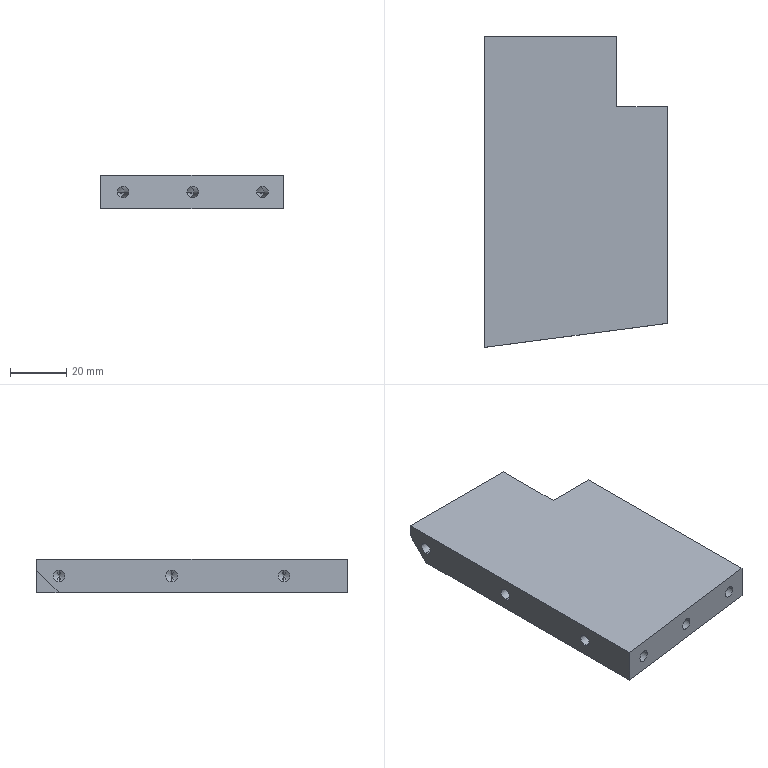Part | SolidWorks | features HoleWzd 4, ICE 3, Extrusion 1 | 1 solid | 46 faces | box 65 x 110.557 x 12 mm | volume 75075 mm3 | cylinder 18 | cone 18 | plane 10 | commonest cylinder face diameters 4.2 x16 4 x2
STEP:
#1=CARTESIAN_POINT('',(6.5,39.5,2.));
#2=VERTEX_POINT('',#1);
#3=CARTESIAN_POINT('',(6.5,39.5,-2.));
#4=VERTEX_POINT('',#3);
#5=CARTESIAN_POINT('',(6.5,39.5,0.));
#6=DIRECTION('',(1.,0.,0.));
#7=DIRECTION('',(0.,0.,-1.));
#8=AXIS2_PLACEMENT_3D('',#5,#6,#7);
#9=CIRCLE('',#8,2.);
#10=EDGE_CURVE('',#2,#4,#9,.T.);
#11=ORIENTED_EDGE('',*,*,#10,.F.);
#12=CARTESIAN_POINT('',(14.5,39.5,2.));
#13=VERTEX_POINT('',#12);
#14=CARTESIAN_POINT('',(14.5,39.5,2.));
#15=DIRECTION('',(1.,0.,0.));
#16=VECTOR('',#15,1000.);
#17=LINE('',#14,#16);
#18=EDGE_CURVE('',#2,#13,#17,.T.);
#19=ORIENTED_EDGE('',*,*,#18,.T.);
#20=CARTESIAN_POINT('',(14.5,39.5,-2.));
#21=VERTEX_POINT('',#20);
#22=CARTESIAN_POINT('',(14.5,39.5,0.));
#23=DIRECTION('',(1.,0.,0.));
#24=DIRECTION('',(0.,0.,-1.));
#25=AXIS2_PLACEMENT_3D('',#22,#23,#24);
#26=CIRCLE('',#25,2.);
#27=EDGE_CURVE('',#13,#21,#26,.T.);
#28=ORIENTED_EDGE('',*,*,#27,.T.);
#29=CARTESIAN_POINT('',(14.5,39.5,-2.));
#30=DIRECTION('',(1.,0.,0.));
#31=VECTOR('',#30,1000.);
#32=LINE('',#29,#31);
#33=EDGE_CURVE('',#4,#21,#32,.T.);
#34=ORIENTED_EDGE('',*,*,#33,.F.);
#35=EDGE_LOOP('',(#11,#19,#28,#34));
#36=FACE_OUTER_BOUND('',#35,.T.);
#37=CARTESIAN_POINT('',(14.5,39.5,0.));
#38=DIRECTION('',(1.,0.,0.));
#39=DIRECTION('',(0.,0.,-1.));
#40=AXIS2_PLACEMENT_3D('',#37,#38,#39);
#41=CYLINDRICAL_SURFACE('',#40,2.);
#42=ADVANCED_FACE('',(#36),#41,.F.);
#43=CARTESIAN_POINT('',(5.298,39.5,0.));
#44=VERTEX_POINT('',#43);
#45=CARTESIAN_POINT('',(6.5,39.5,-2.));
#46=DIRECTION('',(0.515,0.,-0.8572));
#47=VECTOR('',#46,1000.);
#48=LINE('',#45,#47);
#49=EDGE_CURVE('',#44,#4,#48,.T.);
#50=ORIENTED_EDGE('',*,*,#49,.F.);
#51=CARTESIAN_POINT('',(6.5,39.5,2.));
#52=DIRECTION('',(0.515,0.,0.8572));
#53=VECTOR('',#52,1000.);
#54=LINE('',#51,#53);
#55=EDGE_CURVE('',#44,#2,#54,.T.);
#56=ORIENTED_EDGE('',*,*,#55,.T.);
#57=ORIENTED_EDGE('',*,*,#10,.T.);
#58=EDGE_LOOP('',(#50,#56,#57));
#59=FACE_OUTER_BOUND('',#58,.T.);
#60=CARTESIAN_POINT('',(6.5,39.5,0.));
#61=DIRECTION('',(1.,0.,0.));
#62=DIRECTION('',(0.,0.,-1.));
#63=AXIS2_PLACEMENT_3D('',#60,#61,#62);
#64=CONICAL_SURFACE('',#63,2.,1.03);
#65=ADVANCED_FACE('',(#59),#64,.F.);
#66=CARTESIAN_POINT('',(2.1,47.,2.1));
#67=VERTEX_POINT('',#66);
#68=CARTESIAN_POINT('',(2.1,47.,-2.1));
#69=VERTEX_POINT('',#68);
#70=CARTESIAN_POINT('',(2.1,47.,0.));
#71=DIRECTION('',(1.,0.,0.));
#72=DIRECTION('',(0.,0.,-1.));
#73=AXIS2_PLACEMENT_3D('',#70,#71,#72);
#74=CIRCLE('',#73,2.1);
#75=EDGE_CURVE('',#67,#69,#74,.T.);
#76=ORIENTED_EDGE('',*,*,#75,.F.);
#77=CARTESIAN_POINT('',(14.5,47.,2.1));
#78=VERTEX_POINT('',#77);
#79=CARTESIAN_POINT('',(14.5,47.,2.1));
#80=DIRECTION('',(1.,0.,0.));
#81=VECTOR('',#80,1000.);
#82=LINE('',#79,#81);
#83=EDGE_CURVE('',#67,#78,#82,.T.);
#84=ORIENTED_EDGE('',*,*,#83,.T.);
#85=CARTESIAN_POINT('',(14.5,47.,-2.1));
#86=VERTEX_POINT('',#85);
#87=CARTESIAN_POINT('',(14.5,47.,0.));
#88=DIRECTION('',(1.,0.,0.));
#89=DIRECTION('',(0.,0.,-1.));
#90=AXIS2_PLACEMENT_3D('',#87,#88,#89);
#91=CIRCLE('',#90,2.1);
#92=EDGE_CURVE('',#78,#86,#91,.T.);
#93=ORIENTED_EDGE('',*,*,#92,.T.);
#94=CARTESIAN_POINT('',(14.5,47.,-2.1));
#95=DIRECTION('',(1.,0.,0.));
#96=VECTOR('',#95,1000.);
#97=LINE('',#94,#96);
#98=EDGE_CURVE('',#69,#86,#97,.T.);
#99=ORIENTED_EDGE('',*,*,#98,.F.);
#100=EDGE_LOOP('',(#76,#84,#93,#99));
#101=FACE_OUTER_BOUND('',#100,.T.);
#102=CARTESIAN_POINT('',(14.5,47.,0.));
#103=DIRECTION('',(1.,0.,0.));
#104=DIRECTION('',(0.,0.,-1.));
#105=AXIS2_PLACEMENT_3D('',#102,#103,#104);
#106=CYLINDRICAL_SURFACE('',#105,2.1);
#107=ADVANCED_FACE('',(#101),#106,.F.);
#108=CARTESIAN_POINT('',(0.8382,47.,0.));
#109=VERTEX_POINT('',#108);
#110=CARTESIAN_POINT('',(2.1,47.,-2.1));
#111=DIRECTION('',(0.515,0.,-0.8572));
#112=VECTOR('',#111,1000.);
#113=LINE('',#110,#112);
#114=EDGE_CURVE('',#109,#69,#113,.T.);
#115=ORIENTED_EDGE('',*,*,#114,.F.);
#116=CARTESIAN_POINT('',(2.1,47.,2.1));
#117=DIRECTION('',(0.515,0.,0.8572));
#118=VECTOR('',#117,1000.);
#119=LINE('',#116,#118);
#120=EDGE_CURVE('',#109,#67,#119,.T.);
#121=ORIENTED_EDGE('',*,*,#120,.T.);
#122=ORIENTED_EDGE('',*,*,#75,.T.);
#123=EDGE_LOOP('',(#115,#121,#122));
#124=FACE_OUTER_BOUND('',#123,.T.);
#125=CARTESIAN_POINT('',(2.1,47.,0.));
#126=DIRECTION('',(1.,0.,0.));
#127=DIRECTION('',(0.,0.,-1.));
#128=AXIS2_PLACEMENT_3D('',#125,#126,#127);
#129=CONICAL_SURFACE('',#128,2.1,1.03);
#130=ADVANCED_FACE('',(#124),#129,.F.);
#131=CARTESIAN_POINT('',(2.1,32.,2.1));
#132=VERTEX_POINT('',#131);
#133=CARTESIAN_POINT('',(2.1,32.,-2.1));
#134=VERTEX_POINT('',#133);
#135=CARTESIAN_POINT('',(2.1,32.,0.));
#136=DIRECTION('',(1.,0.,0.));
#137=DIRECTION('',(0.,0.,-1.));
#138=AXIS2_PLACEMENT_3D('',#135,#136,#137);
#139=CIRCLE('',#138,2.1);
#140=EDGE_CURVE('',#132,#134,#139,.T.);
#141=ORIENTED_EDGE('',*,*,#140,.F.);
#142=CARTESIAN_POINT('',(14.5,32.,2.1));
#143=VERTEX_POINT('',#142);
#144=CARTESIAN_POINT('',(14.5,32.,2.1));
#145=DIRECTION('',(1.,0.,0.));
#146=VECTOR('',#145,1000.);
#147=LINE('',#144,#146);
#148=EDGE_CURVE('',#132,#143,#147,.T.);
#149=ORIENTED_EDGE('',*,*,#148,.T.);
#150=CARTESIAN_POINT('',(14.5,32.,-2.1));
#151=VERTEX_POINT('',#150);
#152=CARTESIAN_POINT('',(14.5,32.,0.));
#153=DIRECTION('',(1.,0.,0.));
#154=DIRECTION('',(0.,0.,-1.));
#155=AXIS2_PLACEMENT_3D('',#152,#153,#154);
#156=CIRCLE('',#155,2.1);
#157=EDGE_CURVE('',#143,#151,#156,.T.);
#158=ORIENTED_EDGE('',*,*,#157,.T.);
#159=CARTESIAN_POINT('',(14.5,32.,-2.1));
#160=DIRECTION('',(1.,0.,0.));
#161=VECTOR('',#160,1000.);
#162=LINE('',#159,#161);
#163=EDGE_CURVE('',#134,#151,#162,.T.);
#164=ORIENTED_EDGE('',*,*,#163,.F.);
#165=EDGE_LOOP('',(#141,#149,#158,#164));
#166=FACE_OUTER_BOUND('',#165,.T.);
#167=CARTESIAN_POINT('',(14.5,32.,0.));
#168=DIRECTION('',(1.,0.,0.));
#169=DIRECTION('',(0.,0.,-1.));
#170=AXIS2_PLACEMENT_3D('',#167,#168,#169);
#171=CYLINDRICAL_SURFACE('',#170,2.1);
#172=ADVANCED_FACE('',(#166),#171,.F.);
#173=CARTESIAN_POINT('',(0.8382,32.,0.));
#174=VERTEX_POINT('',#173);
#175=CARTESIAN_POINT('',(2.1,32.,-2.1));
#176=DIRECTION('',(0.515,0.,-0.8572));
#177=VECTOR('',#176,1000.);
#178=LINE('',#175,#177);
#179=EDGE_CURVE('',#174,#134,#178,.T.);
#180=ORIENTED_EDGE('',*,*,#179,.F.);
#181=CARTESIAN_POINT('',(2.1,32.,2.1));
#182=DIRECTION('',(0.515,0.,0.8572));
#183=VECTOR('',#182,1000.);
#184=LINE('',#181,#183);
#185=EDGE_CURVE('',#174,#132,#184,.T.);
#186=ORIENTED_EDGE('',*,*,#185,.T.);
#187=ORIENTED_EDGE('',*,*,#140,.T.);
#188=EDGE_LOOP('',(#180,#186,#187));
#189=FACE_OUTER_BOUND('',#188,.T.);
#190=CARTESIAN_POINT('',(2.1,32.,0.));
#191=DIRECTION('',(1.,0.,0.));
#192=DIRECTION('',(0.,0.,-1.));
#193=AXIS2_PLACEMENT_3D('',#190,#191,#192);
#194=CONICAL_SURFACE('',#193,2.1,1.03);
#195=ADVANCED_FACE('',(#189),#194,.F.);
#196=CARTESIAN_POINT('',(-20.1,43.,-2.1));
#197=VERTEX_POINT('',#196);
#198=CARTESIAN_POINT('',(-20.1,43.,2.1));
#199=VERTEX_POINT('',#198);
#200=CARTESIAN_POINT('',(-20.1,43.,0.));
#201=DIRECTION('',(-1.,0.,0.));
#202=DIRECTION('',(0.,0.,1.));
#203=AXIS2_PLACEMENT_3D('',#200,#201,#202);
#204=CIRCLE('',#203,2.1);
#205=EDGE_CURVE('',#197,#199,#204,.T.);
#206=ORIENTED_EDGE('',*,*,#205,.F.);
#207=CARTESIAN_POINT('',(-32.5,43.,-2.1));
#208=VERTEX_POINT('',#207);
#209=CARTESIAN_POINT('',(-32.5,43.,-2.1));
#210=DIRECTION('',(-1.,0.,0.));
#211=VECTOR('',#210,1000.);
#212=LINE('',#209,#211);
#213=EDGE_CURVE('',#197,#208,#212,.T.);
#214=ORIENTED_EDGE('',*,*,#213,.T.);
#215=CARTESIAN_POINT('',(-32.5,43.,2.1));
#216=VERTEX_POINT('',#215);
#217=CARTESIAN_POINT('',(-32.5,43.,0.));
#218=DIRECTION('',(-1.,0.,0.));
#219=DIRECTION('',(0.,0.,1.));
#220=AXIS2_PLACEMENT_3D('',#217,#218,#219);
#221=CIRCLE('',#220,2.1);
#222=EDGE_CURVE('',#208,#216,#221,.T.);
#223=ORIENTED_EDGE('',*,*,#222,.T.);
#224=CARTESIAN_POINT('',(-32.5,43.,2.1));
#225=DIRECTION('',(-1.,0.,0.));
#226=VECTOR('',#225,1000.);
#227=LINE('',#224,#226);
#228=EDGE_CURVE('',#199,#216,#227,.T.);
#229=ORIENTED_EDGE('',*,*,#228,.F.);
#230=EDGE_LOOP('',(#206,#214,#223,#229));
#231=FACE_OUTER_BOUND('',#230,.T.);
#232=CARTESIAN_POINT('',(-32.5,43.,0.));
#233=DIRECTION('',(-1.,0.,0.));
#234=DIRECTION('',(0.,0.,1.));
#235=AXIS2_PLACEMENT_3D('',#232,#233,#234);
#236=CYLINDRICAL_SURFACE('',#235,2.1);
#237=ADVANCED_FACE('',(#231),#236,.F.);
#238=CARTESIAN_POINT('',(-18.838,43.,0.));
#239=VERTEX_POINT('',#238);
#240=CARTESIAN_POINT('',(-20.1,43.,2.1));
#241=DIRECTION('',(-0.515,0.,0.8572));
#242=VECTOR('',#241,1000.);
#243=LINE('',#240,#242);
#244=EDGE_CURVE('',#239,#199,#243,.T.);
#245=ORIENTED_EDGE('',*,*,#244,.F.);
#246=CARTESIAN_POINT('',(-20.1,43.,-2.1));
#247=DIRECTION('',(-0.515,0.,-0.8572));
#248=VECTOR('',#247,1000.);
#249=LINE('',#246,#248);
#250=EDGE_CURVE('',#239,#197,#249,.T.);
#251=ORIENTED_EDGE('',*,*,#250,.T.);
#252=ORIENTED_EDGE('',*,*,#205,.T.);
#253=EDGE_LOOP('',(#245,#251,#252));
#254=FACE_OUTER_BOUND('',#253,.T.);
#255=CARTESIAN_POINT('',(-20.1,43.,0.));
#256=DIRECTION('',(-1.,0.,0.));
#257=DIRECTION('',(0.,0.,1.));
#258=AXIS2_PLACEMENT_3D('',#255,#256,#257);
#259=CONICAL_SURFACE('',#258,2.1,1.03);
#260=ADVANCED_FACE('',(#254),#259,.F.);
#261=CARTESIAN_POINT('',(-20.1,3.,-2.1));
#262=VERTEX_POINT('',#261);
#263=CARTESIAN_POINT('',(-20.1,3.,2.1));
#264=VERTEX_POINT('',#263);
#265=CARTESIAN_POINT('',(-20.1,3.,0.));
#266=DIRECTION('',(-1.,0.,0.));
#267=DIRECTION('',(0.,0.,1.));
#268=AXIS2_PLACEMENT_3D('',#265,#266,#267);
#269=CIRCLE('',#268,2.1);
#270=EDGE_CURVE('',#262,#264,#269,.T.);
#271=ORIENTED_EDGE('',*,*,#270,.F.);
#272=CARTESIAN_POINT('',(-32.5,3.,-2.1));
#273=VERTEX_POINT('',#272);
#274=CARTESIAN_POINT('',(-32.5,3.,-2.1));
#275=DIRECTION('',(-1.,0.,0.));
#276=VECTOR('',#275,1000.);
#277=LINE('',#274,#276);
#278=EDGE_CURVE('',#262,#273,#277,.T.);
#279=ORIENTED_EDGE('',*,*,#278,.T.);
#280=CARTESIAN_POINT('',(-32.5,3.,2.1));
#281=VERTEX_POINT('',#280);
#282=CARTESIAN_POINT('',(-32.5,3.,0.));
#283=DIRECTION('',(-1.,0.,0.));
#284=DIRECTION('',(0.,0.,1.));
#285=AXIS2_PLACEMENT_3D('',#282,#283,#284);
#286=CIRCLE('',#285,2.1);
#287=EDGE_CURVE('',#273,#281,#286,.T.);
#288=ORIENTED_EDGE('',*,*,#287,.T.);
#289=CARTESIAN_POINT('',(-32.5,3.,2.1));
#290=DIRECTION('',(-1.,0.,0.));
#291=VECTOR('',#290,1000.);
#292=LINE('',#289,#291);
#293=EDGE_CURVE('',#264,#281,#292,.T.);
#294=ORIENTED_EDGE('',*,*,#293,.F.);
#295=EDGE_LOOP('',(#271,#279,#288,#294));
#296=FACE_OUTER_BOUND('',#295,.T.);
#297=CARTESIAN_POINT('',(-32.5,3.,0.));
#298=DIRECTION('',(-1.,0.,0.));
#299=DIRECTION('',(0.,0.,1.));
#300=AXIS2_PLACEMENT_3D('',#297,#298,#299);
#301=CYLINDRICAL_SURFACE('',#300,2.1);
#302=ADVANCED_FACE('',(#296),#301,.F.);
#303=CARTESIAN_POINT('',(-18.838,3.,0.));
#304=VERTEX_POINT('',#303);
#305=CARTESIAN_POINT('',(-20.1,3.,2.1));
#306=DIRECTION('',(-0.515,0.,0.8572));
#307=VECTOR('',#306,1000.);
#308=LINE('',#305,#307);
#309=EDGE_CURVE('',#304,#264,#308,.T.);
#310=ORIENTED_EDGE('',*,*,#309,.F.);
#311=CARTESIAN_POINT('',(-20.1,3.,-2.1));
#312=DIRECTION('',(-0.515,0.,-0.8572));
#313=VECTOR('',#312,1000.);
#314=LINE('',#311,#313);
#315=EDGE_CURVE('',#304,#262,#314,.T.);
#316=ORIENTED_EDGE('',*,*,#315,.T.);
#317=ORIENTED_EDGE('',*,*,#270,.T.);
#318=EDGE_LOOP('',(#310,#316,#317));
#319=FACE_OUTER_BOUND('',#318,.T.);
#320=CARTESIAN_POINT('',(-20.1,3.,0.));
#321=DIRECTION('',(-1.,0.,0.));
#322=DIRECTION('',(0.,0.,1.));
#323=AXIS2_PLACEMENT_3D('',#320,#321,#322);
#324=CONICAL_SURFACE('',#323,2.1,1.03);
#325=ADVANCED_FACE('',(#319),#324,.F.);
#326=CARTESIAN_POINT('',(-20.1,-37.,-2.1));
#327=VERTEX_POINT('',#326);
#328=CARTESIAN_POINT('',(-20.1,-37.,2.1));
#329=VERTEX_POINT('',#328);
#330=CARTESIAN_POINT('',(-20.1,-37.,0.));
#331=DIRECTION('',(-1.,0.,0.));
#332=DIRECTION('',(0.,0.,1.));
#333=AXIS2_PLACEMENT_3D('',#330,#331,#332);
#334=CIRCLE('',#333,2.1);
#335=EDGE_CURVE('',#327,#329,#334,.T.);
#336=ORIENTED_EDGE('',*,*,#335,.F.);
#337=CARTESIAN_POINT('',(-32.5,-37.,-2.1));
#338=VERTEX_POINT('',#337);
#339=CARTESIAN_POINT('',(-32.5,-37.,-2.1));
#340=DIRECTION('',(-1.,0.,0.));
#341=VECTOR('',#340,1000.);
#342=LINE('',#339,#341);
#343=EDGE_CURVE('',#327,#338,#342,.T.);
#344=ORIENTED_EDGE('',*,*,#343,.T.);
#345=CARTESIAN_POINT('',(-32.5,-37.,2.1));
#346=VERTEX_POINT('',#345);
#347=CARTESIAN_POINT('',(-32.5,-37.,0.));
#348=DIRECTION('',(-1.,0.,0.));
#349=DIRECTION('',(0.,0.,1.));
#350=AXIS2_PLACEMENT_3D('',#347,#348,#349);
#351=CIRCLE('',#350,2.1);
#352=EDGE_CURVE('',#338,#346,#351,.T.);
#353=ORIENTED_EDGE('',*,*,#352,.T.);
#354=CARTESIAN_POINT('',(-32.5,-37.,2.1));
#355=DIRECTION('',(-1.,0.,0.));
#356=VECTOR('',#355,1000.);
#357=LINE('',#354,#356);
#358=EDGE_CURVE('',#329,#346,#357,.T.);
#359=ORIENTED_EDGE('',*,*,#358,.F.);
#360=EDGE_LOOP('',(#336,#344,#353,#359));
#361=FACE_OUTER_BOUND('',#360,.T.);
#362=CARTESIAN_POINT('',(-32.5,-37.,0.));
#363=DIRECTION('',(-1.,0.,0.));
#364=DIRECTION('',(0.,0.,1.));
#365=AXIS2_PLACEMENT_3D('',#362,#363,#364);
#366=CYLINDRICAL_SURFACE('',#365,2.1);
#367=ADVANCED_FACE('',(#361),#366,.F.);
#368=CARTESIAN_POINT('',(-18.838,-37.,0.));
#369=VERTEX_POINT('',#368);
#370=CARTESIAN_POINT('',(-20.1,-37.,2.1));
#371=DIRECTION('',(-0.515,0.,0.8572));
#372=VECTOR('',#371,1000.);
#373=LINE('',#370,#372);
#374=EDGE_CURVE('',#369,#329,#373,.T.);
#375=ORIENTED_EDGE('',*,*,#374,.F.);
#376=CARTESIAN_POINT('',(-20.1,-37.,-2.1));
#377=DIRECTION('',(-0.515,0.,-0.8572));
#378=VECTOR('',#377,1000.);
#379=LINE('',#376,#378);
#380=EDGE_CURVE('',#369,#327,#379,.T.);
#381=ORIENTED_EDGE('',*,*,#380,.T.);
#382=ORIENTED_EDGE('',*,*,#335,.T.);
#383=EDGE_LOOP('',(#375,#381,#382));
#384=FACE_OUTER_BOUND('',#383,.T.);
#385=CARTESIAN_POINT('',(-20.1,-37.,0.));
#386=DIRECTION('',(-1.,0.,0.));
#387=DIRECTION('',(0.,0.,1.));
#388=AXIS2_PLACEMENT_3D('',#385,#386,#387);
#389=CONICAL_SURFACE('',#388,2.1,1.03);
#390=ADVANCED_FACE('',(#384),#389,.F.);
#391=CARTESIAN_POINT('',(21.364,-39.959,0.));
#392=VERTEX_POINT('',#391);
#393=CARTESIAN_POINT('',(25.528,-39.411,0.));
#394=VERTEX_POINT('',#393);
#395=CARTESIAN_POINT('',(23.446,-39.685,0.));
#396=DIRECTION('',(0.1305,-0.9914,0.));
#397=DIRECTION('',(0.9914,0.1305,0.));
#398=AXIS2_PLACEMENT_3D('',#395,#396,#397);
#399=CIRCLE('',#398,2.1);
#400=EDGE_CURVE('',#392,#394,#399,.T.);
#401=ORIENTED_EDGE('',*,*,#400,.F.);
#402=CARTESIAN_POINT('',(22.982,-52.253,0.));
#403=VERTEX_POINT('',#402);
#404=CARTESIAN_POINT('',(22.982,-52.253,0.));
#405=DIRECTION('',(0.1305,-0.9914,0.));
#406=VECTOR('',#405,1000.);
#407=LINE('',#404,#406);
#408=EDGE_CURVE('',#392,#403,#407,.T.);
#409=ORIENTED_EDGE('',*,*,#408,.T.);
#410=CARTESIAN_POINT('',(27.146,-51.705,0.));
#411=VERTEX_POINT('',#410);
#412=CARTESIAN_POINT('',(25.064,-51.979,0.));
#413=DIRECTION('',(0.1305,-0.9914,0.));
#414=DIRECTION('',(0.9914,0.1305,0.));
#415=AXIS2_PLACEMENT_3D('',#412,#413,#414);
#416=CIRCLE('',#415,2.1);
#417=EDGE_CURVE('',#403,#411,#416,.T.);
#418=ORIENTED_EDGE('',*,*,#417,.T.);
#419=CARTESIAN_POINT('',(27.146,-51.705,0.));
#420=DIRECTION('',(0.1305,-0.9914,0.));
#421=VECTOR('',#420,1000.);
#422=LINE('',#419,#421);
#423=EDGE_CURVE('',#394,#411,#422,.T.);
#424=ORIENTED_EDGE('',*,*,#423,.F.);
#425=EDGE_LOOP('',(#401,#409,#418,#424));
#426=FACE_OUTER_BOUND('',#425,.T.);
#427=CARTESIAN_POINT('',(25.064,-51.979,0.));
#428=DIRECTION('',(0.1305,-0.9914,0.));
#429=DIRECTION('',(0.9914,0.1305,0.));
#430=AXIS2_PLACEMENT_3D('',#427,#428,#429);
#431=CYLINDRICAL_SURFACE('',#430,2.1);
#432=ADVANCED_FACE('',(#426),#431,.F.);
#433=CARTESIAN_POINT('',(23.281,-38.434,0.));
#434=VERTEX_POINT('',#433);
#435=CARTESIAN_POINT('',(25.528,-39.411,0.));
#436=DIRECTION('',(0.9171,-0.3987,0.));
#437=VECTOR('',#436,1000.);
#438=LINE('',#435,#437);
#439=EDGE_CURVE('',#434,#394,#438,.T.);
#440=ORIENTED_EDGE('',*,*,#439,.F.);
#441=CARTESIAN_POINT('',(21.364,-39.959,0.));
#442=DIRECTION('',(-0.7826,-0.6225,0.));
#443=VECTOR('',#442,1000.);
#444=LINE('',#441,#443);
#445=EDGE_CURVE('',#434,#392,#444,.T.);
#446=ORIENTED_EDGE('',*,*,#445,.T.);
#447=ORIENTED_EDGE('',*,*,#400,.T.);
#448=EDGE_LOOP('',(#440,#446,#447));
#449=FACE_OUTER_BOUND('',#448,.T.);
#450=CARTESIAN_POINT('',(23.446,-39.685,0.));
#451=DIRECTION('',(0.1305,-0.9914,0.));
#452=DIRECTION('',(0.9914,0.1305,0.));
#453=AXIS2_PLACEMENT_3D('',#450,#451,#452);
#454=CONICAL_SURFACE('',#453,2.1,1.03);
#455=ADVANCED_FACE('',(#449),#454,.F.);
#456=CARTESIAN_POINT('',(-3.423,-43.222,0.));
#457=VERTEX_POINT('',#456);
#458=CARTESIAN_POINT('',(0.7416,-42.674,0.));
#459=VERTEX_POINT('',#458);
#460=CARTESIAN_POINT('',(-1.34,-42.948,0.));
#461=DIRECTION('',(0.1305,-0.9914,0.));
#462=DIRECTION('',(0.9914,0.1305,0.));
#463=AXIS2_PLACEMENT_3D('',#460,#461,#462);
#464=CIRCLE('',#463,2.1);
#465=EDGE_CURVE('',#457,#459,#464,.T.);
#466=ORIENTED_EDGE('',*,*,#465,.F.);
#467=CARTESIAN_POINT('',(-1.804,-55.516,0.));
#468=VERTEX_POINT('',#467);
#469=CARTESIAN_POINT('',(-1.804,-55.516,0.));
#470=DIRECTION('',(0.1305,-0.9914,0.));
#471=VECTOR('',#470,1000.);
#472=LINE('',#469,#471);
#473=EDGE_CURVE('',#457,#468,#472,.T.);
#474=ORIENTED_EDGE('',*,*,#473,.T.);
#475=CARTESIAN_POINT('',(2.36,-54.968,0.));
#476=VERTEX_POINT('',#475);
#477=CARTESIAN_POINT('',(0.278,-55.242,0.));
#478=DIRECTION('',(0.1305,-0.9914,0.));
#479=DIRECTION('',(0.9914,0.1305,0.));
#480=AXIS2_PLACEMENT_3D('',#477,#478,#479);
#481=CIRCLE('',#480,2.1);
#482=EDGE_CURVE('',#468,#476,#481,.T.);
#483=ORIENTED_EDGE('',*,*,#482,.T.);
#484=CARTESIAN_POINT('',(2.36,-54.968,0.));
#485=DIRECTION('',(0.1305,-0.9914,0.));
#486=VECTOR('',#485,1000.);
#487=LINE('',#484,#486);
#488=EDGE_CURVE('',#459,#476,#487,.T.);
#489=ORIENTED_EDGE('',*,*,#488,.F.);
#490=EDGE_LOOP('',(#466,#474,#483,#489));
#491=FACE_OUTER_BOUND('',#490,.T.);
#492=CARTESIAN_POINT('',(0.278,-55.242,0.));
#493=DIRECTION('',(0.1305,-0.9914,0.));
#494=DIRECTION('',(0.9914,0.1305,0.));
#495=AXIS2_PLACEMENT_3D('',#492,#493,#494);
#496=CYLINDRICAL_SURFACE('',#495,2.1);
#497=ADVANCED_FACE('',(#491),#496,.F.);
#498=CARTESIAN_POINT('',(-1.505,-41.697,0.));
#499=VERTEX_POINT('',#498);
#500=CARTESIAN_POINT('',(0.7416,-42.674,0.));
#501=DIRECTION('',(0.9171,-0.3987,0.));
#502=VECTOR('',#501,1000.);
#503=LINE('',#500,#502);
#504=EDGE_CURVE('',#499,#459,#503,.T.);
#505=ORIENTED_EDGE('',*,*,#504,.F.);
#506=CARTESIAN_POINT('',(-3.423,-43.222,0.));
#507=DIRECTION('',(-0.7826,-0.6225,0.));
#508=VECTOR('',#507,1000.);
#509=LINE('',#506,#508);
#510=EDGE_CURVE('',#499,#457,#509,.T.);
#511=ORIENTED_EDGE('',*,*,#510,.T.);
#512=ORIENTED_EDGE('',*,*,#465,.T.);
#513=EDGE_LOOP('',(#505,#511,#512));
#514=FACE_OUTER_BOUND('',#513,.T.);
#515=CARTESIAN_POINT('',(-1.34,-42.948,0.));
#516=DIRECTION('',(0.1305,-0.9914,0.));
#517=DIRECTION('',(0.9914,0.1305,0.));
#518=AXIS2_PLACEMENT_3D('',#515,#516,#517);
#519=CONICAL_SURFACE('',#518,2.1,1.03);
#520=ADVANCED_FACE('',(#514),#519,.F.);
#521=CARTESIAN_POINT('',(-28.209,-46.485,0.));
#522=VERTEX_POINT('',#521);
#523=CARTESIAN_POINT('',(-24.045,-45.937,0.));
#524=VERTEX_POINT('',#523);
#525=CARTESIAN_POINT('',(-26.127,-46.211,0.));
#526=DIRECTION('',(0.1305,-0.9914,0.));
#527=DIRECTION('',(0.9914,0.1305,0.));
#528=AXIS2_PLACEMENT_3D('',#525,#526,#527);
#529=CIRCLE('',#528,2.1);
#530=EDGE_CURVE('',#522,#524,#529,.T.);
#531=ORIENTED_EDGE('',*,*,#530,.F.);
#532=CARTESIAN_POINT('',(-26.59,-58.779,0.));
#533=VERTEX_POINT('',#532);
#534=CARTESIAN_POINT('',(-26.59,-58.779,0.));
#535=DIRECTION('',(0.1305,-0.9914,0.));
#536=VECTOR('',#535,1000.);
#537=LINE('',#534,#536);
#538=EDGE_CURVE('',#522,#533,#537,.T.);
#539=ORIENTED_EDGE('',*,*,#538,.T.);
#540=CARTESIAN_POINT('',(-22.426,-58.231,0.));
#541=VERTEX_POINT('',#540);
#542=CARTESIAN_POINT('',(-24.508,-58.505,0.));
#543=DIRECTION('',(0.1305,-0.9914,0.));
#544=DIRECTION('',(0.9914,0.1305,0.));
#545=AXIS2_PLACEMENT_3D('',#542,#543,#544);
#546=CIRCLE('',#545,2.1);
#547=EDGE_CURVE('',#533,#541,#546,.T.);
#548=ORIENTED_EDGE('',*,*,#547,.T.);
#549=CARTESIAN_POINT('',(-22.426,-58.231,0.));
#550=DIRECTION('',(0.1305,-0.9914,0.));
#551=VECTOR('',#550,1000.);
#552=LINE('',#549,#551);
#553=EDGE_CURVE('',#524,#541,#552,.T.);
#554=ORIENTED_EDGE('',*,*,#553,.F.);
#555=EDGE_LOOP('',(#531,#539,#548,#554));
#556=FACE_OUTER_BOUND('',#555,.T.);
#557=CARTESIAN_POINT('',(-24.508,-58.505,0.));
#558=DIRECTION('',(0.1305,-0.9914,0.));
#559=DIRECTION('',(0.9914,0.1305,0.));
#560=AXIS2_PLACEMENT_3D('',#557,#558,#559);
#561=CYLINDRICAL_SURFACE('',#560,2.1);
#562=ADVANCED_FACE('',(#556),#561,.F.);
#563=CARTESIAN_POINT('',(-26.291,-44.96,0.));
#564=VERTEX_POINT('',#563);
#565=CARTESIAN_POINT('',(-24.045,-45.937,0.));
#566=DIRECTION('',(0.9171,-0.3987,0.));
#567=VECTOR('',#566,1000.);
#568=LINE('',#565,#567);
#569=EDGE_CURVE('',#564,#524,#568,.T.);
#570=ORIENTED_EDGE('',*,*,#569,.F.);
#571=CARTESIAN_POINT('',(-28.209,-46.485,0.));
#572=DIRECTION('',(-0.7826,-0.6225,0.));
#573=VECTOR('',#572,1000.);
#574=LINE('',#571,#573);
#575=EDGE_CURVE('',#564,#522,#574,.T.);
#576=ORIENTED_EDGE('',*,*,#575,.T.);
#577=ORIENTED_EDGE('',*,*,#530,.T.);
#578=EDGE_LOOP('',(#570,#576,#577));
#579=FACE_OUTER_BOUND('',#578,.T.);
#580=CARTESIAN_POINT('',(-26.127,-46.211,0.));
#581=DIRECTION('',(0.1305,-0.9914,0.));
#582=DIRECTION('',(0.9914,0.1305,0.));
#583=AXIS2_PLACEMENT_3D('',#580,#581,#582);
#584=CONICAL_SURFACE('',#583,2.1,1.03);
#585=ADVANCED_FACE('',(#579),#584,.F.);
#586=CARTESIAN_POINT('',(32.5,26.,-6.));
#587=VERTEX_POINT('',#586);
#588=CARTESIAN_POINT('',(32.5,-51.,-6.));
#589=VERTEX_POINT('',#588);
#590=CARTESIAN_POINT('',(32.5,51.,-6.));
#591=DIRECTION('',(0.,-1.,0.));
#592=VECTOR('',#591,1000.);
#593=LINE('',#590,#592);
#594=EDGE_CURVE('',#587,#589,#593,.T.);
#595=ORIENTED_EDGE('',*,*,#594,.F.);
#596=CARTESIAN_POINT('',(32.5,26.,6.));
#597=VERTEX_POINT('',#596);
#598=CARTESIAN_POINT('',(32.5,26.,-6.));
#599=DIRECTION('',(0.,0.,1.));
#600=VECTOR('',#599,1000.);
#601=LINE('',#598,#600);
#602=EDGE_CURVE('',#587,#597,#601,.T.);
#603=ORIENTED_EDGE('',*,*,#602,.T.);
#604=CARTESIAN_POINT('',(32.5,-51.,6.));
#605=VERTEX_POINT('',#604);
#606=CARTESIAN_POINT('',(32.5,51.,6.));
#607=DIRECTION('',(0.,-1.,0.));
#608=VECTOR('',#607,1000.);
#609=LINE('',#606,#608);
#610=EDGE_CURVE('',#597,#605,#609,.T.);
#611=ORIENTED_EDGE('',*,*,#610,.T.);
#612=CARTESIAN_POINT('',(32.5,-51.,-6.));
#613=DIRECTION('',(0.,0.,-1.));
#614=VECTOR('',#613,1000.);
#615=LINE('',#612,#614);
#616=EDGE_CURVE('',#605,#589,#615,.T.);
#617=ORIENTED_EDGE('',*,*,#616,.T.);
#618=EDGE_LOOP('',(#595,#603,#611,#617));
#619=FACE_OUTER_BOUND('',#618,.T.);
#620=CARTESIAN_POINT('',(32.5,51.,-6.));
#621=DIRECTION('',(-1.,0.,0.));
#622=DIRECTION('',(0.,0.,1.));
#623=AXIS2_PLACEMENT_3D('',#620,#621,#622);
#624=PLANE('',#623);
#625=ADVANCED_FACE('',(#619),#624,.F.);
#626=CARTESIAN_POINT('',(-32.5,43.,-6.));
#627=VERTEX_POINT('',#626);
#628=CARTESIAN_POINT('',(-32.5,-59.557,-6.));
#629=VERTEX_POINT('',#628);
#630=CARTESIAN_POINT('',(-32.5,51.,-6.));
#631=DIRECTION('',(0.,-1.,0.));
#632=VECTOR('',#631,1000.);
#633=LINE('',#630,#632);
#634=EDGE_CURVE('',#627,#629,#633,.T.);
#635=ORIENTED_EDGE('',*,*,#634,.F.);
#636=CARTESIAN_POINT('',(-4.5,43.,-6.));
#637=VERTEX_POINT('',#636);
#638=CARTESIAN_POINT('',(-4.5,43.,-6.));
#639=DIRECTION('',(-1.,0.,0.));
#640=VECTOR('',#639,1000.);
#641=LINE('',#638,#640);
#642=EDGE_CURVE('',#637,#627,#641,.T.);
#643=ORIENTED_EDGE('',*,*,#642,.F.);
#644=CARTESIAN_POINT('',(-4.5,51.,-6.));
#645=VERTEX_POINT('',#644);
#646=CARTESIAN_POINT('',(-4.5,43.,-6.));
#647=DIRECTION('',(0.,-1.,0.));
#648=VECTOR('',#647,1000.);
#649=LINE('',#646,#648);
#650=EDGE_CURVE('',#645,#637,#649,.T.);
#651=ORIENTED_EDGE('',*,*,#650,.F.);
#652=CARTESIAN_POINT('',(14.5,51.,-6.));
#653=VERTEX_POINT('',#652);
#654=CARTESIAN_POINT('',(-32.5,51.,-6.));
#655=DIRECTION('',(-1.,0.,0.));
#656=VECTOR('',#655,1000.);
#657=LINE('',#654,#656);
#658=EDGE_CURVE('',#653,#645,#657,.T.);
#659=ORIENTED_EDGE('',*,*,#658,.F.);
#660=CARTESIAN_POINT('',(14.5,26.,-6.));
#661=VERTEX_POINT('',#660);
#662=CARTESIAN_POINT('',(14.5,51.,-6.));
#663=DIRECTION('',(0.,-1.,0.));
#664=VECTOR('',#663,1000.);
#665=LINE('',#662,#664);
#666=EDGE_CURVE('',#653,#661,#665,.T.);
#667=ORIENTED_EDGE('',*,*,#666,.T.);
#668=CARTESIAN_POINT('',(32.5,26.,-6.));
#669=DIRECTION('',(1.,0.,0.));
#670=VECTOR('',#669,1000.);
#671=LINE('',#668,#670);
#672=EDGE_CURVE('',#661,#587,#671,.T.);
#673=ORIENTED_EDGE('',*,*,#672,.T.);
#674=ORIENTED_EDGE('',*,*,#594,.T.);
#675=CARTESIAN_POINT('',(32.5,-51.,-6.));
#676=DIRECTION('',(-0.9914,-0.1305,0.));
#677=VECTOR('',#676,1000.);
#678=LINE('',#675,#677);
#679=EDGE_CURVE('',#589,#629,#678,.T.);
#680=ORIENTED_EDGE('',*,*,#679,.T.);
#681=EDGE_LOOP('',(#635,#643,#651,#659,#667,#673,#674,#680));
#682=FACE_OUTER_BOUND('',#681,.T.);
#683=CARTESIAN_POINT('',(-32.5,51.,-6.));
#684=DIRECTION('',(0.,0.,1.));
#685=DIRECTION('',(1.,0.,0.));
#686=AXIS2_PLACEMENT_3D('',#683,#684,#685);
#687=PLANE('',#686);
#688=ADVANCED_FACE('',(#682),#687,.F.);
#689=CARTESIAN_POINT('',(-32.5,43.,0.));
#690=DIRECTION('',(-1.,0.,0.));
#691=DIRECTION('',(0.,0.,1.));
#692=AXIS2_PLACEMENT_3D('',#689,#690,#691);
#693=CIRCLE('',#692,2.1);
#694=EDGE_CURVE('',#216,#208,#693,.T.);
#695=ORIENTED_EDGE('',*,*,#694,.F.);
#696=ORIENTED_EDGE('',*,*,#222,.F.);
#697=EDGE_LOOP('',(#695,#696));
#698=FACE_BOUND('',#697,.T.);
#699=CARTESIAN_POINT('',(-32.5,3.,0.));
#700=DIRECTION('',(-1.,0.,0.));
#701=DIRECTION('',(0.,0.,1.));
#702=AXIS2_PLACEMENT_3D('',#699,#700,#701);
#703=CIRCLE('',#702,2.1);
#704=EDGE_CURVE('',#281,#273,#703,.T.);
#705=ORIENTED_EDGE('',*,*,#704,.F.);
#706=ORIENTED_EDGE('',*,*,#287,.F.);
#707=EDGE_LOOP('',(#705,#706));
#708=FACE_BOUND('',#707,.T.);
#709=CARTESIAN_POINT('',(-32.5,-37.,0.));
#710=DIRECTION('',(-1.,0.,0.));
#711=DIRECTION('',(0.,0.,1.));
#712=AXIS2_PLACEMENT_3D('',#709,#710,#711);
#713=CIRCLE('',#712,2.1);
#714=EDGE_CURVE('',#346,#338,#713,.T.);
#715=ORIENTED_EDGE('',*,*,#714,.F.);
#716=ORIENTED_EDGE('',*,*,#352,.F.);
#717=EDGE_LOOP('',(#715,#716));
#718=FACE_BOUND('',#717,.T.);
#719=CARTESIAN_POINT('',(-32.5,51.,2.));
#720=VERTEX_POINT('',#719);
#721=CARTESIAN_POINT('',(-32.5,51.,6.));
#722=VERTEX_POINT('',#721);
#723=CARTESIAN_POINT('',(-32.5,51.,-6.));
#724=DIRECTION('',(0.,0.,1.));
#725=VECTOR('',#724,1000.);
#726=LINE('',#723,#725);
#727=EDGE_CURVE('',#720,#722,#726,.T.);
#728=ORIENTED_EDGE('',*,*,#727,.F.);
#729=CARTESIAN_POINT('',(-32.5,51.,2.));
#730=DIRECTION('',(0.,0.7071,0.7071));
#731=VECTOR('',#730,1000.);
#732=LINE('',#729,#731);
#733=EDGE_CURVE('',#627,#720,#732,.T.);
#734=ORIENTED_EDGE('',*,*,#733,.F.);
#735=ORIENTED_EDGE('',*,*,#634,.T.);
#736=CARTESIAN_POINT('',(-32.5,-59.557,6.));
#737=VERTEX_POINT('',#736);
#738=CARTESIAN_POINT('',(-32.5,-59.557,-71.561));
#739=DIRECTION('',(0.,0.,1.));
#740=VECTOR('',#739,1000.);
#741=LINE('',#738,#740);
#742=EDGE_CURVE('',#629,#737,#741,.T.);
#743=ORIENTED_EDGE('',*,*,#742,.T.);
#744=CARTESIAN_POINT('',(-32.5,51.,6.));
#745=DIRECTION('',(0.,-1.,0.));
#746=VECTOR('',#745,1000.);
#747=LINE('',#744,#746);
#748=EDGE_CURVE('',#722,#737,#747,.T.);
#749=ORIENTED_EDGE('',*,*,#748,.F.);
#750=EDGE_LOOP('',(#728,#734,#735,#743,#749));
#751=FACE_OUTER_BOUND('',#750,.T.);
#752=CARTESIAN_POINT('',(-32.5,51.,-6.));
#753=DIRECTION('',(1.,0.,0.));
#754=DIRECTION('',(0.,0.,-1.));
#755=AXIS2_PLACEMENT_3D('',#752,#753,#754);
#756=PLANE('',#755);
#757=ADVANCED_FACE('',(#698,#708,#718,#751),#756,.F.);
#758=ORIENTED_EDGE('',*,*,#610,.F.);
#759=CARTESIAN_POINT('',(14.5,26.,6.));
#760=VERTEX_POINT('',#759);
#761=CARTESIAN_POINT('',(32.5,26.,6.));
#762=DIRECTION('',(1.,0.,0.));
#763=VECTOR('',#762,1000.);
#764=LINE('',#761,#763);
#765=EDGE_CURVE('',#760,#597,#764,.T.);
#766=ORIENTED_EDGE('',*,*,#765,.F.);
#767=CARTESIAN_POINT('',(14.5,51.,6.));
#768=VERTEX_POINT('',#767);
#769=CARTESIAN_POINT('',(14.5,51.,6.));
#770=DIRECTION('',(0.,-1.,0.));
#771=VECTOR('',#770,1000.);
#772=LINE('',#769,#771);
#773=EDGE_CURVE('',#768,#760,#772,.T.);
#774=ORIENTED_EDGE('',*,*,#773,.F.);
#775=CARTESIAN_POINT('',(-32.5,51.,6.));
#776=DIRECTION('',(1.,0.,0.));
#777=VECTOR('',#776,1000.);
#778=LINE('',#775,#777);
#779=EDGE_CURVE('',#722,#768,#778,.T.);
#780=ORIENTED_EDGE('',*,*,#779,.F.);
#781=ORIENTED_EDGE('',*,*,#748,.T.);
#782=CARTESIAN_POINT('',(32.5,-51.,6.));
#783=DIRECTION('',(0.9914,0.1305,0.));
#784=VECTOR('',#783,1000.);
#785=LINE('',#782,#784);
#786=EDGE_CURVE('',#737,#605,#785,.T.);
#787=ORIENTED_EDGE('',*,*,#786,.T.);
#788=EDGE_LOOP('',(#758,#766,#774,#780,#781,#787));
#789=FACE_OUTER_BOUND('',#788,.T.);
#790=CARTESIAN_POINT('',(-32.5,51.,6.));
#791=DIRECTION('',(0.,0.,-1.));
#792=DIRECTION('',(-1.,0.,0.));
#793=AXIS2_PLACEMENT_3D('',#790,#791,#792);
#794=PLANE('',#793);
#795=ADVANCED_FACE('',(#789),#794,.F.);
#796=CARTESIAN_POINT('',(-4.5,51.,2.));
#797=VERTEX_POINT('',#796);
#798=CARTESIAN_POINT('',(-4.5,51.,2.));
#799=DIRECTION('',(-1.,0.,0.));
#800=VECTOR('',#799,1000.);
#801=LINE('',#798,#800);
#802=EDGE_CURVE('',#797,#720,#801,.T.);
#803=ORIENTED_EDGE('',*,*,#802,.T.);
#804=ORIENTED_EDGE('',*,*,#727,.T.);
#805=ORIENTED_EDGE('',*,*,#779,.T.);
#806=CARTESIAN_POINT('',(14.5,51.,-6.));
#807=DIRECTION('',(0.,0.,1.));
#808=VECTOR('',#807,1000.);
#809=LINE('',#806,#808);
#810=EDGE_CURVE('',#653,#768,#809,.T.);
#811=ORIENTED_EDGE('',*,*,#810,.F.);
#812=ORIENTED_EDGE('',*,*,#658,.T.);
#813=CARTESIAN_POINT('',(-4.5,51.,-6.));
#814=DIRECTION('',(0.,0.,-1.));
#815=VECTOR('',#814,1000.);
#816=LINE('',#813,#815);
#817=EDGE_CURVE('',#797,#645,#816,.T.);
#818=ORIENTED_EDGE('',*,*,#817,.F.);
#819=EDGE_LOOP('',(#803,#804,#805,#811,#812,#818));
#820=FACE_OUTER_BOUND('',#819,.T.);
#821=CARTESIAN_POINT('',(0.,51.,0.));
#822=DIRECTION('',(0.,1.,0.));
#823=DIRECTION('',(0.,0.,1.));
#824=AXIS2_PLACEMENT_3D('',#821,#822,#823);
#825=PLANE('',#824);
#826=ADVANCED_FACE('',(#820),#825,.T.);
#827=CARTESIAN_POINT('',(25.064,-51.979,0.));
#828=DIRECTION('',(0.1305,-0.9914,0.));
#829=DIRECTION('',(0.9914,0.1305,0.));
#830=AXIS2_PLACEMENT_3D('',#827,#828,#829);
#831=CIRCLE('',#830,2.1);
#832=EDGE_CURVE('',#411,#403,#831,.T.);
#833=ORIENTED_EDGE('',*,*,#832,.F.);
#834=ORIENTED_EDGE('',*,*,#417,.F.);
#835=EDGE_LOOP('',(#833,#834));
#836=FACE_BOUND('',#835,.T.);
#837=CARTESIAN_POINT('',(0.278,-55.242,0.));
#838=DIRECTION('',(0.1305,-0.9914,0.));
#839=DIRECTION('',(0.9914,0.1305,0.));
#840=AXIS2_PLACEMENT_3D('',#837,#838,#839);
#841=CIRCLE('',#840,2.1);
#842=EDGE_CURVE('',#476,#468,#841,.T.);
#843=ORIENTED_EDGE('',*,*,#842,.F.);
#844=ORIENTED_EDGE('',*,*,#482,.F.);
#845=EDGE_LOOP('',(#843,#844));
#846=FACE_BOUND('',#845,.T.);
#847=CARTESIAN_POINT('',(-24.508,-58.505,0.));
#848=DIRECTION('',(0.1305,-0.9914,0.));
#849=DIRECTION('',(0.9914,0.1305,0.));
#850=AXIS2_PLACEMENT_3D('',#847,#848,#849);
#851=CIRCLE('',#850,2.1);
#852=EDGE_CURVE('',#541,#533,#851,.T.);
#853=ORIENTED_EDGE('',*,*,#852,.F.);
#854=ORIENTED_EDGE('',*,*,#547,.F.);
#855=EDGE_LOOP('',(#853,#854));
#856=FACE_BOUND('',#855,.T.);
#857=ORIENTED_EDGE('',*,*,#679,.F.);
#858=ORIENTED_EDGE('',*,*,#616,.F.);
#859=ORIENTED_EDGE('',*,*,#786,.F.);
#860=ORIENTED_EDGE('',*,*,#742,.F.);
#861=EDGE_LOOP('',(#857,#858,#859,#860));
#862=FACE_OUTER_BOUND('',#861,.T.);
#863=CARTESIAN_POINT('',(32.5,-51.,-71.561));
#864=DIRECTION('',(0.1305,-0.9914,0.));
#865=DIRECTION('',(0.9914,0.1305,0.));
#866=AXIS2_PLACEMENT_3D('',#863,#864,#865);
#867=PLANE('',#866);
#868=ADVANCED_FACE('',(#836,#846,#856,#862),#867,.T.);
#869=ORIENTED_EDGE('',*,*,#765,.T.);
#870=ORIENTED_EDGE('',*,*,#602,.F.);
#871=ORIENTED_EDGE('',*,*,#672,.F.);
#872=CARTESIAN_POINT('',(14.5,26.,-6.));
#873=DIRECTION('',(0.,0.,1.));
#874=VECTOR('',#873,1000.);
#875=LINE('',#872,#874);
#876=EDGE_CURVE('',#661,#760,#875,.T.);
#877=ORIENTED_EDGE('',*,*,#876,.T.);
#878=EDGE_LOOP('',(#869,#870,#871,#877));
#879=FACE_OUTER_BOUND('',#878,.T.);
#880=CARTESIAN_POINT('',(32.5,26.,-6.));
#881=DIRECTION('',(0.,-1.,0.));
#882=DIRECTION('',(1.,0.,0.));
#883=AXIS2_PLACEMENT_3D('',#880,#881,#882);
#884=PLANE('',#883);
#885=ADVANCED_FACE('',(#879),#884,.F.);
#886=CARTESIAN_POINT('',(14.5,39.5,0.));
#887=DIRECTION('',(1.,0.,0.));
#888=DIRECTION('',(0.,0.,-1.));
#889=AXIS2_PLACEMENT_3D('',#886,#887,#888);
#890=CIRCLE('',#889,2.);
#891=EDGE_CURVE('',#21,#13,#890,.T.);
#892=ORIENTED_EDGE('',*,*,#891,.F.);
#893=ORIENTED_EDGE('',*,*,#27,.F.);
#894=EDGE_LOOP('',(#892,#893));
#895=FACE_BOUND('',#894,.T.);
#896=CARTESIAN_POINT('',(14.5,47.,0.));
#897=DIRECTION('',(1.,0.,0.));
#898=DIRECTION('',(0.,0.,-1.));
#899=AXIS2_PLACEMENT_3D('',#896,#897,#898);
#900=CIRCLE('',#899,2.1);
#901=EDGE_CURVE('',#86,#78,#900,.T.);
#902=ORIENTED_EDGE('',*,*,#901,.F.);
#903=ORIENTED_EDGE('',*,*,#92,.F.);
#904=EDGE_LOOP('',(#902,#903));
#905=FACE_BOUND('',#904,.T.);
#906=CARTESIAN_POINT('',(14.5,32.,0.));
#907=DIRECTION('',(1.,0.,0.));
#908=DIRECTION('',(0.,0.,-1.));
#909=AXIS2_PLACEMENT_3D('',#906,#907,#908);
#910=CIRCLE('',#909,2.1);
#911=EDGE_CURVE('',#151,#143,#910,.T.);
#912=ORIENTED_EDGE('',*,*,#911,.F.);
#913=ORIENTED_EDGE('',*,*,#157,.F.);
#914=EDGE_LOOP('',(#912,#913));
#915=FACE_BOUND('',#914,.T.);
#916=ORIENTED_EDGE('',*,*,#773,.T.);
#917=ORIENTED_EDGE('',*,*,#876,.F.);
#918=ORIENTED_EDGE('',*,*,#666,.F.);
#919=ORIENTED_EDGE('',*,*,#810,.T.);
#920=EDGE_LOOP('',(#916,#917,#918,#919));
#921=FACE_OUTER_BOUND('',#920,.T.);
#922=CARTESIAN_POINT('',(14.5,51.,-6.));
#923=DIRECTION('',(-1.,0.,0.));
#924=DIRECTION('',(0.,-1.,0.));
#925=AXIS2_PLACEMENT_3D('',#922,#923,#924);
#926=PLANE('',#925);
#927=ADVANCED_FACE('',(#895,#905,#915,#921),#926,.F.);
#928=ORIENTED_EDGE('',*,*,#575,.F.);
#929=ORIENTED_EDGE('',*,*,#569,.T.);
#930=CARTESIAN_POINT('',(-26.127,-46.211,0.));
#931=DIRECTION('',(0.1305,-0.9914,0.));
#932=DIRECTION('',(0.9914,0.1305,0.));
#933=AXIS2_PLACEMENT_3D('',#930,#931,#932);
#934=CIRCLE('',#933,2.1);
#935=EDGE_CURVE('',#524,#522,#934,.T.);
#936=ORIENTED_EDGE('',*,*,#935,.T.);
#937=EDGE_LOOP('',(#928,#929,#936));
#938=FACE_OUTER_BOUND('',#937,.T.);
#939=CARTESIAN_POINT('',(-26.127,-46.211,0.));
#940=DIRECTION('',(0.1305,-0.9914,0.));
#941=DIRECTION('',(0.9914,0.1305,0.));
#942=AXIS2_PLACEMENT_3D('',#939,#940,#941);
#943=CONICAL_SURFACE('',#942,2.1,1.03);
#944=ADVANCED_FACE('',(#938),#943,.F.);
#945=ORIENTED_EDGE('',*,*,#538,.F.);
#946=ORIENTED_EDGE('',*,*,#935,.F.);
#947=ORIENTED_EDGE('',*,*,#553,.T.);
#948=ORIENTED_EDGE('',*,*,#852,.T.);
#949=EDGE_LOOP('',(#945,#946,#947,#948));
#950=FACE_OUTER_BOUND('',#949,.T.);
#951=CARTESIAN_POINT('',(-24.508,-58.505,0.));
#952=DIRECTION('',(0.1305,-0.9914,0.));
#953=DIRECTION('',(0.9914,0.1305,0.));
#954=AXIS2_PLACEMENT_3D('',#951,#952,#953);
#955=CYLINDRICAL_SURFACE('',#954,2.1);
#956=ADVANCED_FACE('',(#950),#955,.F.);
#957=ORIENTED_EDGE('',*,*,#510,.F.);
#958=ORIENTED_EDGE('',*,*,#504,.T.);
#959=CARTESIAN_POINT('',(-1.34,-42.948,0.));
#960=DIRECTION('',(0.1305,-0.9914,0.));
#961=DIRECTION('',(0.9914,0.1305,0.));
#962=AXIS2_PLACEMENT_3D('',#959,#960,#961);
#963=CIRCLE('',#962,2.1);
#964=EDGE_CURVE('',#459,#457,#963,.T.);
#965=ORIENTED_EDGE('',*,*,#964,.T.);
#966=EDGE_LOOP('',(#957,#958,#965));
#967=FACE_OUTER_BOUND('',#966,.T.);
#968=CARTESIAN_POINT('',(-1.34,-42.948,0.));
#969=DIRECTION('',(0.1305,-0.9914,0.));
#970=DIRECTION('',(0.9914,0.1305,0.));
#971=AXIS2_PLACEMENT_3D('',#968,#969,#970);
#972=CONICAL_SURFACE('',#971,2.1,1.03);
#973=ADVANCED_FACE('',(#967),#972,.F.);
#974=ORIENTED_EDGE('',*,*,#473,.F.);
#975=ORIENTED_EDGE('',*,*,#964,.F.);
#976=ORIENTED_EDGE('',*,*,#488,.T.);
#977=ORIENTED_EDGE('',*,*,#842,.T.);
#978=EDGE_LOOP('',(#974,#975,#976,#977));
#979=FACE_OUTER_BOUND('',#978,.T.);
#980=CARTESIAN_POINT('',(0.278,-55.242,0.));
#981=DIRECTION('',(0.1305,-0.9914,0.));
#982=DIRECTION('',(0.9914,0.1305,0.));
#983=AXIS2_PLACEMENT_3D('',#980,#981,#982);
#984=CYLINDRICAL_SURFACE('',#983,2.1);
#985=ADVANCED_FACE('',(#979),#984,.F.);
#986=ORIENTED_EDGE('',*,*,#445,.F.);
#987=ORIENTED_EDGE('',*,*,#439,.T.);
#988=CARTESIAN_POINT('',(23.446,-39.685,0.));
#989=DIRECTION('',(0.1305,-0.9914,0.));
#990=DIRECTION('',(0.9914,0.1305,0.));
#991=AXIS2_PLACEMENT_3D('',#988,#989,#990);
#992=CIRCLE('',#991,2.1);
#993=EDGE_CURVE('',#394,#392,#992,.T.);
#994=ORIENTED_EDGE('',*,*,#993,.T.);
#995=EDGE_LOOP('',(#986,#987,#994));
#996=FACE_OUTER_BOUND('',#995,.T.);
#997=CARTESIAN_POINT('',(23.446,-39.685,0.));
#998=DIRECTION('',(0.1305,-0.9914,0.));
#999=DIRECTION('',(0.9914,0.1305,0.));
#1000=AXIS2_PLACEMENT_3D('',#997,#998,#999);
#1001=CONICAL_SURFACE('',#1000,2.1,1.03);
#1002=ADVANCED_FACE('',(#996),#1001,.F.);
#1003=ORIENTED_EDGE('',*,*,#408,.F.);
#1004=ORIENTED_EDGE('',*,*,#993,.F.);
#1005=ORIENTED_EDGE('',*,*,#423,.T.);
#1006=ORIENTED_EDGE('',*,*,#832,.T.);
#1007=EDGE_LOOP('',(#1003,#1004,#1005,#1006));
#1008=FACE_OUTER_BOUND('',#1007,.T.);
#1009=CARTESIAN_POINT('',(25.064,-51.979,0.));
#1010=DIRECTION('',(0.1305,-0.9914,0.));
#1011=DIRECTION('',(0.9914,0.1305,0.));
#1012=AXIS2_PLACEMENT_3D('',#1009,#1010,#1011);
#1013=CYLINDRICAL_SURFACE('',#1012,2.1);
#1014=ADVANCED_FACE('',(#1008),#1013,.F.);
#1015=ORIENTED_EDGE('',*,*,#380,.F.);
#1016=ORIENTED_EDGE('',*,*,#374,.T.);
#1017=CARTESIAN_POINT('',(-20.1,-37.,0.));
#1018=DIRECTION('',(-1.,0.,0.));
#1019=DIRECTION('',(0.,0.,1.));
#1020=AXIS2_PLACEMENT_3D('',#1017,#1018,#1019);
#1021=CIRCLE('',#1020,2.1);
#1022=EDGE_CURVE('',#329,#327,#1021,.T.);
#1023=ORIENTED_EDGE('',*,*,#1022,.T.);
#1024=EDGE_LOOP('',(#1015,#1016,#1023));
#1025=FACE_OUTER_BOUND('',#1024,.T.);
#1026=CARTESIAN_POINT('',(-20.1,-37.,0.));
#1027=DIRECTION('',(-1.,0.,0.));
#1028=DIRECTION('',(0.,0.,1.));
#1029=AXIS2_PLACEMENT_3D('',#1026,#1027,#1028);
#1030=CONICAL_SURFACE('',#1029,2.1,1.03);
#1031=ADVANCED_FACE('',(#1025),#1030,.F.);
#1032=ORIENTED_EDGE('',*,*,#343,.F.);
#1033=ORIENTED_EDGE('',*,*,#1022,.F.);
#1034=ORIENTED_EDGE('',*,*,#358,.T.);
#1035=ORIENTED_EDGE('',*,*,#714,.T.);
#1036=EDGE_LOOP('',(#1032,#1033,#1034,#1035));
#1037=FACE_OUTER_BOUND('',#1036,.T.);
#1038=CARTESIAN_POINT('',(-32.5,-37.,0.));
#1039=DIRECTION('',(-1.,0.,0.));
#1040=DIRECTION('',(0.,0.,1.));
#1041=AXIS2_PLACEMENT_3D('',#1038,#1039,#1040);
#1042=CYLINDRICAL_SURFACE('',#1041,2.1);
#1043=ADVANCED_FACE('',(#1037),#1042,.F.);
#1044=ORIENTED_EDGE('',*,*,#315,.F.);
#1045=ORIENTED_EDGE('',*,*,#309,.T.);
#1046=CARTESIAN_POINT('',(-20.1,3.,0.));
#1047=DIRECTION('',(-1.,0.,0.));
#1048=DIRECTION('',(0.,0.,1.));
#1049=AXIS2_PLACEMENT_3D('',#1046,#1047,#1048);
#1050=CIRCLE('',#1049,2.1);
#1051=EDGE_CURVE('',#264,#262,#1050,.T.);
#1052=ORIENTED_EDGE('',*,*,#1051,.T.);
#1053=EDGE_LOOP('',(#1044,#1045,#1052));
#1054=FACE_OUTER_BOUND('',#1053,.T.);
#1055=CARTESIAN_POINT('',(-20.1,3.,0.));
#1056=DIRECTION('',(-1.,0.,0.));
#1057=DIRECTION('',(0.,0.,1.));
#1058=AXIS2_PLACEMENT_3D('',#1055,#1056,#1057);
#1059=CONICAL_SURFACE('',#1058,2.1,1.03);
#1060=ADVANCED_FACE('',(#1054),#1059,.F.);
#1061=ORIENTED_EDGE('',*,*,#278,.F.);
#1062=ORIENTED_EDGE('',*,*,#1051,.F.);
#1063=ORIENTED_EDGE('',*,*,#293,.T.);
#1064=ORIENTED_EDGE('',*,*,#704,.T.);
#1065=EDGE_LOOP('',(#1061,#1062,#1063,#1064));
#1066=FACE_OUTER_BOUND('',#1065,.T.);
#1067=CARTESIAN_POINT('',(-32.5,3.,0.));
#1068=DIRECTION('',(-1.,0.,0.));
#1069=DIRECTION('',(0.,0.,1.));
#1070=AXIS2_PLACEMENT_3D('',#1067,#1068,#1069);
#1071=CYLINDRICAL_SURFACE('',#1070,2.1);
#1072=ADVANCED_FACE('',(#1066),#1071,.F.);
#1073=ORIENTED_EDGE('',*,*,#250,.F.);
#1074=ORIENTED_EDGE('',*,*,#244,.T.);
#1075=CARTESIAN_POINT('',(-20.1,43.,0.));
#1076=DIRECTION('',(-1.,0.,0.));
#1077=DIRECTION('',(0.,0.,1.));
#1078=AXIS2_PLACEMENT_3D('',#1075,#1076,#1077);
#1079=CIRCLE('',#1078,2.1);
#1080=EDGE_CURVE('',#199,#197,#1079,.T.);
#1081=ORIENTED_EDGE('',*,*,#1080,.T.);
#1082=EDGE_LOOP('',(#1073,#1074,#1081));
#1083=FACE_OUTER_BOUND('',#1082,.T.);
#1084=CARTESIAN_POINT('',(-20.1,43.,0.));
#1085=DIRECTION('',(-1.,0.,0.));
#1086=DIRECTION('',(0.,0.,1.));
#1087=AXIS2_PLACEMENT_3D('',#1084,#1085,#1086);
#1088=CONICAL_SURFACE('',#1087,2.1,1.03);
#1089=ADVANCED_FACE('',(#1083),#1088,.F.);
#1090=ORIENTED_EDGE('',*,*,#213,.F.);
#1091=ORIENTED_EDGE('',*,*,#1080,.F.);
#1092=ORIENTED_EDGE('',*,*,#228,.T.);
#1093=ORIENTED_EDGE('',*,*,#694,.T.);
#1094=EDGE_LOOP('',(#1090,#1091,#1092,#1093));
#1095=FACE_OUTER_BOUND('',#1094,.T.);
#1096=CARTESIAN_POINT('',(-32.5,43.,0.));
#1097=DIRECTION('',(-1.,0.,0.));
#1098=DIRECTION('',(0.,0.,1.));
#1099=AXIS2_PLACEMENT_3D('',#1096,#1097,#1098);
#1100=CYLINDRICAL_SURFACE('',#1099,2.1);
#1101=ADVANCED_FACE('',(#1095),#1100,.F.);
#1102=ORIENTED_EDGE('',*,*,#185,.F.);
#1103=ORIENTED_EDGE('',*,*,#179,.T.);
#1104=CARTESIAN_POINT('',(2.1,32.,0.));
#1105=DIRECTION('',(1.,0.,0.));
#1106=DIRECTION('',(0.,0.,-1.));
#1107=AXIS2_PLACEMENT_3D('',#1104,#1105,#1106);
#1108=CIRCLE('',#1107,2.1);
#1109=EDGE_CURVE('',#134,#132,#1108,.T.);
#1110=ORIENTED_EDGE('',*,*,#1109,.T.);
#1111=EDGE_LOOP('',(#1102,#1103,#1110));
#1112=FACE_OUTER_BOUND('',#1111,.T.);
#1113=CARTESIAN_POINT('',(2.1,32.,0.));
#1114=DIRECTION('',(1.,0.,0.));
#1115=DIRECTION('',(0.,0.,-1.));
#1116=AXIS2_PLACEMENT_3D('',#1113,#1114,#1115);
#1117=CONICAL_SURFACE('',#1116,2.1,1.03);
#1118=ADVANCED_FACE('',(#1112),#1117,.F.);
#1119=ORIENTED_EDGE('',*,*,#148,.F.);
#1120=ORIENTED_EDGE('',*,*,#1109,.F.);
#1121=ORIENTED_EDGE('',*,*,#163,.T.);
#1122=ORIENTED_EDGE('',*,*,#911,.T.);
#1123=EDGE_LOOP('',(#1119,#1120,#1121,#1122));
#1124=FACE_OUTER_BOUND('',#1123,.T.);
#1125=CARTESIAN_POINT('',(14.5,32.,0.));
#1126=DIRECTION('',(1.,0.,0.));
#1127=DIRECTION('',(0.,0.,-1.));
#1128=AXIS2_PLACEMENT_3D('',#1125,#1126,#1127);
#1129=CYLINDRICAL_SURFACE('',#1128,2.1);
#1130=ADVANCED_FACE('',(#1124),#1129,.F.);
#1131=ORIENTED_EDGE('',*,*,#120,.F.);
#1132=ORIENTED_EDGE('',*,*,#114,.T.);
#1133=CARTESIAN_POINT('',(2.1,47.,0.));
#1134=DIRECTION('',(1.,0.,0.));
#1135=DIRECTION('',(0.,0.,-1.));
#1136=AXIS2_PLACEMENT_3D('',#1133,#1134,#1135);
#1137=CIRCLE('',#1136,2.1);
#1138=EDGE_CURVE('',#69,#67,#1137,.T.);
#1139=ORIENTED_EDGE('',*,*,#1138,.T.);
#1140=EDGE_LOOP('',(#1131,#1132,#1139));
#1141=FACE_OUTER_BOUND('',#1140,.T.);
#1142=CARTESIAN_POINT('',(2.1,47.,0.));
#1143=DIRECTION('',(1.,0.,0.));
#1144=DIRECTION('',(0.,0.,-1.));
#1145=AXIS2_PLACEMENT_3D('',#1142,#1143,#1144);
#1146=CONICAL_SURFACE('',#1145,2.1,1.03);
#1147=ADVANCED_FACE('',(#1141),#1146,.F.);
#1148=ORIENTED_EDGE('',*,*,#83,.F.);
#1149=ORIENTED_EDGE('',*,*,#1138,.F.);
#1150=ORIENTED_EDGE('',*,*,#98,.T.);
#1151=ORIENTED_EDGE('',*,*,#901,.T.);
#1152=EDGE_LOOP('',(#1148,#1149,#1150,#1151));
#1153=FACE_OUTER_BOUND('',#1152,.T.);
#1154=CARTESIAN_POINT('',(14.5,47.,0.));
#1155=DIRECTION('',(1.,0.,0.));
#1156=DIRECTION('',(0.,0.,-1.));
#1157=AXIS2_PLACEMENT_3D('',#1154,#1155,#1156);
#1158=CYLINDRICAL_SURFACE('',#1157,2.1);
#1159=ADVANCED_FACE('',(#1153),#1158,.F.);
#1160=ORIENTED_EDGE('',*,*,#733,.T.);
#1161=ORIENTED_EDGE('',*,*,#802,.F.);
#1162=CARTESIAN_POINT('',(-4.5,51.,2.));
#1163=DIRECTION('',(0.,0.7071,0.7071));
#1164=VECTOR('',#1163,1000.);
#1165=LINE('',#1162,#1164);
#1166=EDGE_CURVE('',#637,#797,#1165,.T.);
#1167=ORIENTED_EDGE('',*,*,#1166,.F.);
#1168=ORIENTED_EDGE('',*,*,#642,.T.);
#1169=EDGE_LOOP('',(#1160,#1161,#1167,#1168));
#1170=FACE_OUTER_BOUND('',#1169,.T.);
#1171=CARTESIAN_POINT('',(-4.5,51.,2.));
#1172=DIRECTION('',(0.,-0.7071,0.7071));
#1173=DIRECTION('',(0.,-0.7071,-0.7071));
#1174=AXIS2_PLACEMENT_3D('',#1171,#1172,#1173);
#1175=PLANE('',#1174);
#1176=ADVANCED_FACE('',(#1170),#1175,.F.);
#1177=ORIENTED_EDGE('',*,*,#1166,.T.);
#1178=ORIENTED_EDGE('',*,*,#817,.T.);
#1179=ORIENTED_EDGE('',*,*,#650,.T.);
#1180=EDGE_LOOP('',(#1177,#1178,#1179));
#1181=FACE_OUTER_BOUND('',#1180,.T.);
#1182=CARTESIAN_POINT('',(-4.5,0.,0.));
#1183=DIRECTION('',(1.,0.,0.));
#1184=DIRECTION('',(0.,0.,-1.));
#1185=AXIS2_PLACEMENT_3D('',#1182,#1183,#1184);
#1186=PLANE('',#1185);
#1187=ADVANCED_FACE('',(#1181),#1186,.F.);
#1188=ORIENTED_EDGE('',*,*,#55,.F.);
#1189=ORIENTED_EDGE('',*,*,#49,.T.);
#1190=CARTESIAN_POINT('',(6.5,39.5,0.));
#1191=DIRECTION('',(1.,0.,0.));
#1192=DIRECTION('',(0.,0.,-1.));
#1193=AXIS2_PLACEMENT_3D('',#1190,#1191,#1192);
#1194=CIRCLE('',#1193,2.);
#1195=EDGE_CURVE('',#4,#2,#1194,.T.);
#1196=ORIENTED_EDGE('',*,*,#1195,.T.);
#1197=EDGE_LOOP('',(#1188,#1189,#1196));
#1198=FACE_OUTER_BOUND('',#1197,.T.);
#1199=CARTESIAN_POINT('',(6.5,39.5,0.));
#1200=DIRECTION('',(1.,0.,0.));
#1201=DIRECTION('',(0.,0.,-1.));
#1202=AXIS2_PLACEMENT_3D('',#1199,#1200,#1201);
#1203=CONICAL_SURFACE('',#1202,2.,1.03);
#1204=ADVANCED_FACE('',(#1198),#1203,.F.);
#1205=ORIENTED_EDGE('',*,*,#18,.F.);
#1206=ORIENTED_EDGE('',*,*,#1195,.F.);
#1207=ORIENTED_EDGE('',*,*,#33,.T.);
#1208=ORIENTED_EDGE('',*,*,#891,.T.);
#1209=EDGE_LOOP('',(#1205,#1206,#1207,#1208));
#1210=FACE_OUTER_BOUND('',#1209,.T.);
#1211=CARTESIAN_POINT('',(14.5,39.5,0.));
#1212=DIRECTION('',(1.,0.,0.));
#1213=DIRECTION('',(0.,0.,-1.));
#1214=AXIS2_PLACEMENT_3D('',#1211,#1212,#1213);
#1215=CYLINDRICAL_SURFACE('',#1214,2.);
#1216=ADVANCED_FACE('',(#1210),#1215,.F.);
#1217=CLOSED_SHELL('',(#42,#65,#107,#130,#172,#195,#237,#260,#302,#325,#367,#390,#432,#455,#497,#520,#562,#585,#625,#688,#757,#795,#826,#868,#885,#927,#944,#956,#973,#985,#1002,#1014,#1031,#1043,#1060,#1072,#1089,#1101,#1118,#1130,#1147,#1159,#1176,#1187,#1204,#1216));
#1218=MANIFOLD_SOLID_BREP('',#1217);
#1219=CARTESIAN_POINT('',(0.,0.,0.));
#1220=DIRECTION('',(0.,0.,1.));
#1221=DIRECTION('',(1.,0.,0.));
#1222=AXIS2_PLACEMENT_3D('',#1219,#1220,#1221);
#1223=(LENGTH_UNIT()NAMED_UNIT(*)SI_UNIT(.MILLI.,.METRE.));
#1224=UNCERTAINTY_MEASURE_WITH_UNIT(LENGTH_MEASURE(0.00001),#1223,'','');
#1225=(NAMED_UNIT(*)PLANE_ANGLE_UNIT()SI_UNIT($,.RADIAN.));
#1226=(NAMED_UNIT(*)SI_UNIT($,.STERADIAN.)SOLID_ANGLE_UNIT());
#1227=(GEOMETRIC_REPRESENTATION_CONTEXT(3)GLOBAL_UNCERTAINTY_ASSIGNED_CONTEXT((#1224))GLOBAL_UNIT_ASSIGNED_CONTEXT((#1223,#1225,#1226))REPRESENTATION_CONTEXT('',''));
#1228=ADVANCED_BREP_SHAPE_REPRESENTATION('',(#1218,#1222),#1227);